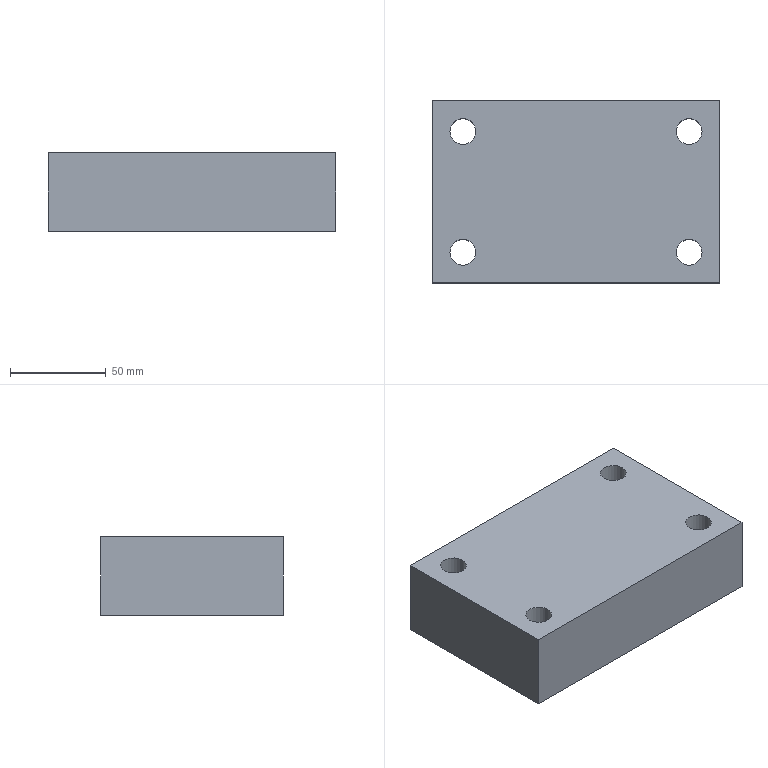Part | NX | features solid 2 | 1 solid | 18 faces | box 150 x 95 x 41 mm | volume 550514 mm3 | plane 10 | cylinder 8 | commonest cylinder face diameters 13.5 x4 20 x4
STEP:
#1=CARTESIAN_POINT('',(1702.045,-31.5,60.));
#2=VERTEX_POINT('',#1);
#3=CARTESIAN_POINT('',(1692.045,-31.5,60.));
#4=DIRECTION('',(0.,0.,1.));
#5=DIRECTION('',(1.,0.,0.));
#6=AXIS2_PLACEMENT_3D('',#3,#4,#5);
#7=CIRCLE('',#6,10.);
#8=EDGE_CURVE('',#2,#2,#7,.T.);
#9=ORIENTED_EDGE('',*,*,#8,.T.);
#10=EDGE_LOOP('',(#9));
#11=FACE_BOUND('',#10,.T.);
#12=CARTESIAN_POINT('',(1584.045,31.5,60.));
#13=VERTEX_POINT('',#12);
#14=CARTESIAN_POINT('',(1574.045,31.5,60.));
#15=DIRECTION('',(0.,0.,1.));
#16=DIRECTION('',(1.,0.,0.));
#17=AXIS2_PLACEMENT_3D('',#14,#15,#16);
#18=CIRCLE('',#17,10.);
#19=EDGE_CURVE('',#13,#13,#18,.T.);
#20=ORIENTED_EDGE('',*,*,#19,.T.);
#21=EDGE_LOOP('',(#20));
#22=FACE_BOUND('',#21,.T.);
#23=CARTESIAN_POINT('',(1708.045,-47.5,60.));
#24=VERTEX_POINT('',#23);
#25=CARTESIAN_POINT('',(1708.045,47.5,60.));
#26=VERTEX_POINT('',#25);
#27=CARTESIAN_POINT('',(1708.045,0.,60.));
#28=DIRECTION('',(0.,1.,0.));
#29=VECTOR('',#28,1000.);
#30=LINE('',#27,#29);
#31=EDGE_CURVE('',#24,#26,#30,.T.);
#32=ORIENTED_EDGE('',*,*,#31,.F.);
#33=CARTESIAN_POINT('',(1558.045,-47.5,60.));
#34=VERTEX_POINT('',#33);
#35=CARTESIAN_POINT('',(1633.045,-47.5,60.));
#36=DIRECTION('',(1.,0.,0.));
#37=VECTOR('',#36,1000.);
#38=LINE('',#35,#37);
#39=EDGE_CURVE('',#34,#24,#38,.T.);
#40=ORIENTED_EDGE('',*,*,#39,.F.);
#41=CARTESIAN_POINT('',(1558.045,47.5,60.));
#42=VERTEX_POINT('',#41);
#43=CARTESIAN_POINT('',(1558.045,0.,60.));
#44=DIRECTION('',(0.,-1.,0.));
#45=VECTOR('',#44,1000.);
#46=LINE('',#43,#45);
#47=EDGE_CURVE('',#42,#34,#46,.T.);
#48=ORIENTED_EDGE('',*,*,#47,.F.);
#49=CARTESIAN_POINT('',(1633.045,47.5,60.));
#50=DIRECTION('',(-1.,0.,0.));
#51=VECTOR('',#50,1000.);
#52=LINE('',#49,#51);
#53=EDGE_CURVE('',#26,#42,#52,.T.);
#54=ORIENTED_EDGE('',*,*,#53,.F.);
#55=EDGE_LOOP('',(#32,#40,#48,#54));
#56=FACE_BOUND('',#55,.T.);
#57=CARTESIAN_POINT('',(1584.045,-31.5,60.));
#58=VERTEX_POINT('',#57);
#59=CARTESIAN_POINT('',(1574.045,-31.5,60.));
#60=DIRECTION('',(0.,0.,1.));
#61=DIRECTION('',(1.,0.,0.));
#62=AXIS2_PLACEMENT_3D('',#59,#60,#61);
#63=CIRCLE('',#62,10.);
#64=EDGE_CURVE('',#58,#58,#63,.T.);
#65=ORIENTED_EDGE('',*,*,#64,.T.);
#66=EDGE_LOOP('',(#65));
#67=FACE_BOUND('',#66,.T.);
#68=CARTESIAN_POINT('',(1702.045,31.5,60.));
#69=VERTEX_POINT('',#68);
#70=CARTESIAN_POINT('',(1692.045,31.5,60.));
#71=DIRECTION('',(0.,0.,1.));
#72=DIRECTION('',(1.,0.,0.));
#73=AXIS2_PLACEMENT_3D('',#70,#71,#72);
#74=CIRCLE('',#73,10.);
#75=EDGE_CURVE('',#69,#69,#74,.T.);
#76=ORIENTED_EDGE('',*,*,#75,.T.);
#77=EDGE_LOOP('',(#76));
#78=FACE_BOUND('',#77,.T.);
#79=CARTESIAN_POINT('',(1633.045,0.,60.));
#80=DIRECTION('',(0.,0.,-1.));
#81=DIRECTION('',(1.,0.,0.));
#82=AXIS2_PLACEMENT_3D('',#79,#80,#81);
#83=PLANE('',#82);
#84=ADVANCED_FACE('',(#11,#22,#56,#67,#78),#83,.T.);
#85=CARTESIAN_POINT('',(1698.795,31.5,101.));
#86=VERTEX_POINT('',#85);
#87=CARTESIAN_POINT('',(1692.045,31.5,101.));
#88=DIRECTION('',(0.,0.,1.));
#89=DIRECTION('',(1.,0.,0.));
#90=AXIS2_PLACEMENT_3D('',#87,#88,#89);
#91=CIRCLE('',#90,6.75);
#92=EDGE_CURVE('',#86,#86,#91,.T.);
#93=ORIENTED_EDGE('',*,*,#92,.F.);
#94=EDGE_LOOP('',(#93));
#95=FACE_BOUND('',#94,.T.);
#96=CARTESIAN_POINT('',(1698.795,-31.5,101.));
#97=VERTEX_POINT('',#96);
#98=CARTESIAN_POINT('',(1692.045,-31.5,101.));
#99=DIRECTION('',(0.,0.,1.));
#100=DIRECTION('',(1.,0.,0.));
#101=AXIS2_PLACEMENT_3D('',#98,#99,#100);
#102=CIRCLE('',#101,6.75);
#103=EDGE_CURVE('',#97,#97,#102,.T.);
#104=ORIENTED_EDGE('',*,*,#103,.F.);
#105=EDGE_LOOP('',(#104));
#106=FACE_BOUND('',#105,.T.);
#107=CARTESIAN_POINT('',(1580.795,-31.5,101.));
#108=VERTEX_POINT('',#107);
#109=CARTESIAN_POINT('',(1574.045,-31.5,101.));
#110=DIRECTION('',(0.,0.,1.));
#111=DIRECTION('',(1.,0.,0.));
#112=AXIS2_PLACEMENT_3D('',#109,#110,#111);
#113=CIRCLE('',#112,6.75);
#114=EDGE_CURVE('',#108,#108,#113,.T.);
#115=ORIENTED_EDGE('',*,*,#114,.F.);
#116=EDGE_LOOP('',(#115));
#117=FACE_BOUND('',#116,.T.);
#118=CARTESIAN_POINT('',(1580.795,31.5,101.));
#119=VERTEX_POINT('',#118);
#120=CARTESIAN_POINT('',(1574.045,31.5,101.));
#121=DIRECTION('',(0.,0.,1.));
#122=DIRECTION('',(1.,0.,0.));
#123=AXIS2_PLACEMENT_3D('',#120,#121,#122);
#124=CIRCLE('',#123,6.75);
#125=EDGE_CURVE('',#119,#119,#124,.T.);
#126=ORIENTED_EDGE('',*,*,#125,.F.);
#127=EDGE_LOOP('',(#126));
#128=FACE_BOUND('',#127,.T.);
#129=CARTESIAN_POINT('',(1708.045,-47.5,101.));
#130=VERTEX_POINT('',#129);
#131=CARTESIAN_POINT('',(1558.045,-47.5,101.));
#132=VERTEX_POINT('',#131);
#133=CARTESIAN_POINT('',(1633.045,-47.5,101.));
#134=DIRECTION('',(-1.,0.,0.));
#135=VECTOR('',#134,1000.);
#136=LINE('',#133,#135);
#137=EDGE_CURVE('',#130,#132,#136,.T.);
#138=ORIENTED_EDGE('',*,*,#137,.F.);
#139=CARTESIAN_POINT('',(1708.045,47.5,101.));
#140=VERTEX_POINT('',#139);
#141=CARTESIAN_POINT('',(1708.045,0.,101.));
#142=DIRECTION('',(0.,-1.,0.));
#143=VECTOR('',#142,1000.);
#144=LINE('',#141,#143);
#145=EDGE_CURVE('',#140,#130,#144,.T.);
#146=ORIENTED_EDGE('',*,*,#145,.F.);
#147=CARTESIAN_POINT('',(1558.045,47.5,101.));
#148=VERTEX_POINT('',#147);
#149=CARTESIAN_POINT('',(1633.045,47.5,101.));
#150=DIRECTION('',(1.,0.,0.));
#151=VECTOR('',#150,1000.);
#152=LINE('',#149,#151);
#153=EDGE_CURVE('',#148,#140,#152,.T.);
#154=ORIENTED_EDGE('',*,*,#153,.F.);
#155=CARTESIAN_POINT('',(1558.045,0.,101.));
#156=DIRECTION('',(0.,1.,0.));
#157=VECTOR('',#156,1000.);
#158=LINE('',#155,#157);
#159=EDGE_CURVE('',#132,#148,#158,.T.);
#160=ORIENTED_EDGE('',*,*,#159,.F.);
#161=EDGE_LOOP('',(#138,#146,#154,#160));
#162=FACE_BOUND('',#161,.T.);
#163=CARTESIAN_POINT('',(1633.045,0.,101.));
#164=DIRECTION('',(0.,0.,1.));
#165=DIRECTION('',(-1.,0.,0.));
#166=AXIS2_PLACEMENT_3D('',#163,#164,#165);
#167=PLANE('',#166);
#168=ADVANCED_FACE('',(#95,#106,#117,#128,#162),#167,.T.);
#169=CARTESIAN_POINT('',(1708.045,-47.5,81.));
#170=DIRECTION('',(0.,0.,1.));
#171=VECTOR('',#170,1000.);
#172=LINE('',#169,#171);
#173=EDGE_CURVE('',#24,#130,#172,.T.);
#174=ORIENTED_EDGE('',*,*,#173,.T.);
#175=ORIENTED_EDGE('',*,*,#137,.T.);
#176=CARTESIAN_POINT('',(1558.045,-47.5,81.));
#177=DIRECTION('',(0.,0.,1.));
#178=VECTOR('',#177,1000.);
#179=LINE('',#176,#178);
#180=EDGE_CURVE('',#34,#132,#179,.T.);
#181=ORIENTED_EDGE('',*,*,#180,.F.);
#182=ORIENTED_EDGE('',*,*,#39,.T.);
#183=EDGE_LOOP('',(#174,#175,#181,#182));
#184=FACE_BOUND('',#183,.T.);
#185=CARTESIAN_POINT('',(1633.045,-47.5,81.));
#186=DIRECTION('',(0.,-1.,0.));
#187=DIRECTION('',(0.,0.,1.));
#188=AXIS2_PLACEMENT_3D('',#185,#186,#187);
#189=PLANE('',#188);
#190=ADVANCED_FACE('',(#184),#189,.T.);
#191=ORIENTED_EDGE('',*,*,#180,.T.);
#192=ORIENTED_EDGE('',*,*,#159,.T.);
#193=CARTESIAN_POINT('',(1558.045,47.5,81.));
#194=DIRECTION('',(0.,0.,1.));
#195=VECTOR('',#194,1000.);
#196=LINE('',#193,#195);
#197=EDGE_CURVE('',#42,#148,#196,.T.);
#198=ORIENTED_EDGE('',*,*,#197,.F.);
#199=ORIENTED_EDGE('',*,*,#47,.T.);
#200=EDGE_LOOP('',(#191,#192,#198,#199));
#201=FACE_BOUND('',#200,.T.);
#202=CARTESIAN_POINT('',(1558.045,0.,81.));
#203=DIRECTION('',(-1.,0.,0.));
#204=DIRECTION('',(0.,0.,-1.));
#205=AXIS2_PLACEMENT_3D('',#202,#203,#204);
#206=PLANE('',#205);
#207=ADVANCED_FACE('',(#201),#206,.T.);
#208=ORIENTED_EDGE('',*,*,#197,.T.);
#209=ORIENTED_EDGE('',*,*,#153,.T.);
#210=CARTESIAN_POINT('',(1708.045,47.5,81.));
#211=DIRECTION('',(0.,0.,1.));
#212=VECTOR('',#211,1000.);
#213=LINE('',#210,#212);
#214=EDGE_CURVE('',#26,#140,#213,.T.);
#215=ORIENTED_EDGE('',*,*,#214,.F.);
#216=ORIENTED_EDGE('',*,*,#53,.T.);
#217=EDGE_LOOP('',(#208,#209,#215,#216));
#218=FACE_BOUND('',#217,.T.);
#219=CARTESIAN_POINT('',(1633.045,47.5,81.));
#220=DIRECTION('',(0.,1.,0.));
#221=DIRECTION('',(0.,0.,-1.));
#222=AXIS2_PLACEMENT_3D('',#219,#220,#221);
#223=PLANE('',#222);
#224=ADVANCED_FACE('',(#218),#223,.T.);
#225=ORIENTED_EDGE('',*,*,#31,.T.);
#226=ORIENTED_EDGE('',*,*,#214,.T.);
#227=ORIENTED_EDGE('',*,*,#145,.T.);
#228=ORIENTED_EDGE('',*,*,#173,.F.);
#229=EDGE_LOOP('',(#225,#226,#227,#228));
#230=FACE_BOUND('',#229,.T.);
#231=CARTESIAN_POINT('',(1708.045,0.,81.));
#232=DIRECTION('',(1.,0.,0.));
#233=DIRECTION('',(0.,0.,1.));
#234=AXIS2_PLACEMENT_3D('',#231,#232,#233);
#235=PLANE('',#234);
#236=ADVANCED_FACE('',(#230),#235,.T.);
#237=ORIENTED_EDGE('',*,*,#125,.T.);
#238=EDGE_LOOP('',(#237));
#239=FACE_BOUND('',#238,.T.);
#240=CARTESIAN_POINT('',(1580.795,31.5,75.));
#241=VERTEX_POINT('',#240);
#242=CARTESIAN_POINT('',(1574.045,31.5,75.));
#243=DIRECTION('',(0.,0.,1.));
#244=DIRECTION('',(1.,0.,0.));
#245=AXIS2_PLACEMENT_3D('',#242,#243,#244);
#246=CIRCLE('',#245,6.75);
#247=EDGE_CURVE('',#241,#241,#246,.T.);
#248=ORIENTED_EDGE('',*,*,#247,.F.);
#249=EDGE_LOOP('',(#248));
#250=FACE_BOUND('',#249,.T.);
#251=CARTESIAN_POINT('',(1574.045,31.5,55.));
#252=DIRECTION('',(0.,0.,1.));
#253=DIRECTION('',(-1.,0.,0.));
#254=AXIS2_PLACEMENT_3D('',#251,#252,#253);
#255=CYLINDRICAL_SURFACE('',#254,6.75);
#256=ADVANCED_FACE('',(#239,#250),#255,.F.);
#257=ORIENTED_EDGE('',*,*,#247,.T.);
#258=EDGE_LOOP('',(#257));
#259=FACE_BOUND('',#258,.T.);
#260=CARTESIAN_POINT('',(1584.045,31.5,75.));
#261=VERTEX_POINT('',#260);
#262=CARTESIAN_POINT('',(1574.045,31.5,75.));
#263=DIRECTION('',(0.,0.,1.));
#264=DIRECTION('',(1.,0.,0.));
#265=AXIS2_PLACEMENT_3D('',#262,#263,#264);
#266=CIRCLE('',#265,10.);
#267=EDGE_CURVE('',#261,#261,#266,.T.);
#268=ORIENTED_EDGE('',*,*,#267,.F.);
#269=EDGE_LOOP('',(#268));
#270=FACE_BOUND('',#269,.T.);
#271=CARTESIAN_POINT('',(1574.045,31.5,75.));
#272=DIRECTION('',(0.,0.,1.));
#273=DIRECTION('',(-1.,0.,0.));
#274=AXIS2_PLACEMENT_3D('',#271,#272,#273);
#275=PLANE('',#274);
#276=ADVANCED_FACE('',(#259,#270),#275,.F.);
#277=ORIENTED_EDGE('',*,*,#267,.T.);
#278=EDGE_LOOP('',(#277));
#279=FACE_BOUND('',#278,.T.);
#280=ORIENTED_EDGE('',*,*,#19,.F.);
#281=EDGE_LOOP('',(#280));
#282=FACE_BOUND('',#281,.T.);
#283=CARTESIAN_POINT('',(1574.045,31.5,60.));
#284=DIRECTION('',(0.,0.,1.));
#285=DIRECTION('',(-1.,0.,0.));
#286=AXIS2_PLACEMENT_3D('',#283,#284,#285);
#287=CYLINDRICAL_SURFACE('',#286,10.);
#288=ADVANCED_FACE('',(#279,#282),#287,.F.);
#289=ORIENTED_EDGE('',*,*,#114,.T.);
#290=EDGE_LOOP('',(#289));
#291=FACE_BOUND('',#290,.T.);
#292=CARTESIAN_POINT('',(1580.795,-31.5,75.));
#293=VERTEX_POINT('',#292);
#294=CARTESIAN_POINT('',(1574.045,-31.5,75.));
#295=DIRECTION('',(0.,0.,1.));
#296=DIRECTION('',(1.,0.,0.));
#297=AXIS2_PLACEMENT_3D('',#294,#295,#296);
#298=CIRCLE('',#297,6.75);
#299=EDGE_CURVE('',#293,#293,#298,.T.);
#300=ORIENTED_EDGE('',*,*,#299,.F.);
#301=EDGE_LOOP('',(#300));
#302=FACE_BOUND('',#301,.T.);
#303=CARTESIAN_POINT('',(1574.045,-31.5,55.));
#304=DIRECTION('',(0.,0.,1.));
#305=DIRECTION('',(-1.,0.,0.));
#306=AXIS2_PLACEMENT_3D('',#303,#304,#305);
#307=CYLINDRICAL_SURFACE('',#306,6.75);
#308=ADVANCED_FACE('',(#291,#302),#307,.F.);
#309=ORIENTED_EDGE('',*,*,#299,.T.);
#310=EDGE_LOOP('',(#309));
#311=FACE_BOUND('',#310,.T.);
#312=CARTESIAN_POINT('',(1584.045,-31.5,75.));
#313=VERTEX_POINT('',#312);
#314=CARTESIAN_POINT('',(1574.045,-31.5,75.));
#315=DIRECTION('',(0.,0.,1.));
#316=DIRECTION('',(1.,0.,0.));
#317=AXIS2_PLACEMENT_3D('',#314,#315,#316);
#318=CIRCLE('',#317,10.);
#319=EDGE_CURVE('',#313,#313,#318,.T.);
#320=ORIENTED_EDGE('',*,*,#319,.F.);
#321=EDGE_LOOP('',(#320));
#322=FACE_BOUND('',#321,.T.);
#323=CARTESIAN_POINT('',(1574.045,-31.5,75.));
#324=DIRECTION('',(0.,0.,1.));
#325=DIRECTION('',(-1.,0.,0.));
#326=AXIS2_PLACEMENT_3D('',#323,#324,#325);
#327=PLANE('',#326);
#328=ADVANCED_FACE('',(#311,#322),#327,.F.);
#329=ORIENTED_EDGE('',*,*,#319,.T.);
#330=EDGE_LOOP('',(#329));
#331=FACE_BOUND('',#330,.T.);
#332=ORIENTED_EDGE('',*,*,#64,.F.);
#333=EDGE_LOOP('',(#332));
#334=FACE_BOUND('',#333,.T.);
#335=CARTESIAN_POINT('',(1574.045,-31.5,60.));
#336=DIRECTION('',(0.,0.,1.));
#337=DIRECTION('',(-1.,0.,0.));
#338=AXIS2_PLACEMENT_3D('',#335,#336,#337);
#339=CYLINDRICAL_SURFACE('',#338,10.);
#340=ADVANCED_FACE('',(#331,#334),#339,.F.);
#341=ORIENTED_EDGE('',*,*,#103,.T.);
#342=EDGE_LOOP('',(#341));
#343=FACE_BOUND('',#342,.T.);
#344=CARTESIAN_POINT('',(1698.795,-31.5,75.));
#345=VERTEX_POINT('',#344);
#346=CARTESIAN_POINT('',(1692.045,-31.5,75.));
#347=DIRECTION('',(0.,0.,1.));
#348=DIRECTION('',(1.,0.,0.));
#349=AXIS2_PLACEMENT_3D('',#346,#347,#348);
#350=CIRCLE('',#349,6.75);
#351=EDGE_CURVE('',#345,#345,#350,.T.);
#352=ORIENTED_EDGE('',*,*,#351,.F.);
#353=EDGE_LOOP('',(#352));
#354=FACE_BOUND('',#353,.T.);
#355=CARTESIAN_POINT('',(1692.045,-31.5,55.));
#356=DIRECTION('',(0.,0.,1.));
#357=DIRECTION('',(-1.,0.,0.));
#358=AXIS2_PLACEMENT_3D('',#355,#356,#357);
#359=CYLINDRICAL_SURFACE('',#358,6.75);
#360=ADVANCED_FACE('',(#343,#354),#359,.F.);
#361=ORIENTED_EDGE('',*,*,#351,.T.);
#362=EDGE_LOOP('',(#361));
#363=FACE_BOUND('',#362,.T.);
#364=CARTESIAN_POINT('',(1702.045,-31.5,75.));
#365=VERTEX_POINT('',#364);
#366=CARTESIAN_POINT('',(1692.045,-31.5,75.));
#367=DIRECTION('',(0.,0.,1.));
#368=DIRECTION('',(1.,0.,0.));
#369=AXIS2_PLACEMENT_3D('',#366,#367,#368);
#370=CIRCLE('',#369,10.);
#371=EDGE_CURVE('',#365,#365,#370,.T.);
#372=ORIENTED_EDGE('',*,*,#371,.F.);
#373=EDGE_LOOP('',(#372));
#374=FACE_BOUND('',#373,.T.);
#375=CARTESIAN_POINT('',(1692.045,-31.5,75.));
#376=DIRECTION('',(0.,0.,1.));
#377=DIRECTION('',(-1.,0.,0.));
#378=AXIS2_PLACEMENT_3D('',#375,#376,#377);
#379=PLANE('',#378);
#380=ADVANCED_FACE('',(#363,#374),#379,.F.);
#381=ORIENTED_EDGE('',*,*,#371,.T.);
#382=EDGE_LOOP('',(#381));
#383=FACE_BOUND('',#382,.T.);
#384=ORIENTED_EDGE('',*,*,#8,.F.);
#385=EDGE_LOOP('',(#384));
#386=FACE_BOUND('',#385,.T.);
#387=CARTESIAN_POINT('',(1692.045,-31.5,60.));
#388=DIRECTION('',(0.,0.,1.));
#389=DIRECTION('',(-1.,0.,0.));
#390=AXIS2_PLACEMENT_3D('',#387,#388,#389);
#391=CYLINDRICAL_SURFACE('',#390,10.);
#392=ADVANCED_FACE('',(#383,#386),#391,.F.);
#393=ORIENTED_EDGE('',*,*,#92,.T.);
#394=EDGE_LOOP('',(#393));
#395=FACE_BOUND('',#394,.T.);
#396=CARTESIAN_POINT('',(1698.795,31.5,75.));
#397=VERTEX_POINT('',#396);
#398=CARTESIAN_POINT('',(1692.045,31.5,75.));
#399=DIRECTION('',(0.,0.,1.));
#400=DIRECTION('',(1.,0.,0.));
#401=AXIS2_PLACEMENT_3D('',#398,#399,#400);
#402=CIRCLE('',#401,6.75);
#403=EDGE_CURVE('',#397,#397,#402,.T.);
#404=ORIENTED_EDGE('',*,*,#403,.F.);
#405=EDGE_LOOP('',(#404));
#406=FACE_BOUND('',#405,.T.);
#407=CARTESIAN_POINT('',(1692.045,31.5,55.));
#408=DIRECTION('',(0.,0.,1.));
#409=DIRECTION('',(-1.,0.,0.));
#410=AXIS2_PLACEMENT_3D('',#407,#408,#409);
#411=CYLINDRICAL_SURFACE('',#410,6.75);
#412=ADVANCED_FACE('',(#395,#406),#411,.F.);
#413=ORIENTED_EDGE('',*,*,#403,.T.);
#414=EDGE_LOOP('',(#413));
#415=FACE_BOUND('',#414,.T.);
#416=CARTESIAN_POINT('',(1702.045,31.5,75.));
#417=VERTEX_POINT('',#416);
#418=CARTESIAN_POINT('',(1692.045,31.5,75.));
#419=DIRECTION('',(0.,0.,1.));
#420=DIRECTION('',(1.,0.,0.));
#421=AXIS2_PLACEMENT_3D('',#418,#419,#420);
#422=CIRCLE('',#421,10.);
#423=EDGE_CURVE('',#417,#417,#422,.T.);
#424=ORIENTED_EDGE('',*,*,#423,.F.);
#425=EDGE_LOOP('',(#424));
#426=FACE_BOUND('',#425,.T.);
#427=CARTESIAN_POINT('',(1692.045,31.5,75.));
#428=DIRECTION('',(0.,0.,1.));
#429=DIRECTION('',(-1.,0.,0.));
#430=AXIS2_PLACEMENT_3D('',#427,#428,#429);
#431=PLANE('',#430);
#432=ADVANCED_FACE('',(#415,#426),#431,.F.);
#433=ORIENTED_EDGE('',*,*,#423,.T.);
#434=EDGE_LOOP('',(#433));
#435=FACE_BOUND('',#434,.T.);
#436=ORIENTED_EDGE('',*,*,#75,.F.);
#437=EDGE_LOOP('',(#436));
#438=FACE_BOUND('',#437,.T.);
#439=CARTESIAN_POINT('',(1692.045,31.5,60.));
#440=DIRECTION('',(0.,0.,1.));
#441=DIRECTION('',(-1.,0.,0.));
#442=AXIS2_PLACEMENT_3D('',#439,#440,#441);
#443=CYLINDRICAL_SURFACE('',#442,10.);
#444=ADVANCED_FACE('',(#435,#438),#443,.F.);
#445=CLOSED_SHELL('',(#84,#168,#190,#207,#224,#236,#256,#276,#288,#308,#328,#340,#360,#380,#392,#412,#432,#444));
#446=MANIFOLD_SOLID_BREP('',#445);
#447=(LENGTH_UNIT()NAMED_UNIT(*)SI_UNIT(.MILLI.,.METRE.));
#448=UNCERTAINTY_MEASURE_WITH_UNIT(LENGTH_MEASURE(0.00001),#447,'','');
#449=(NAMED_UNIT(*)PLANE_ANGLE_UNIT()SI_UNIT($,.RADIAN.));
#450=(NAMED_UNIT(*)SI_UNIT($,.STERADIAN.)SOLID_ANGLE_UNIT());
#451=(GEOMETRIC_REPRESENTATION_CONTEXT(3)GLOBAL_UNCERTAINTY_ASSIGNED_CONTEXT((#448))GLOBAL_UNIT_ASSIGNED_CONTEXT((#447,#449,#450))REPRESENTATION_CONTEXT('',''));
#452=ADVANCED_BREP_SHAPE_REPRESENTATION('',(#446),#451);